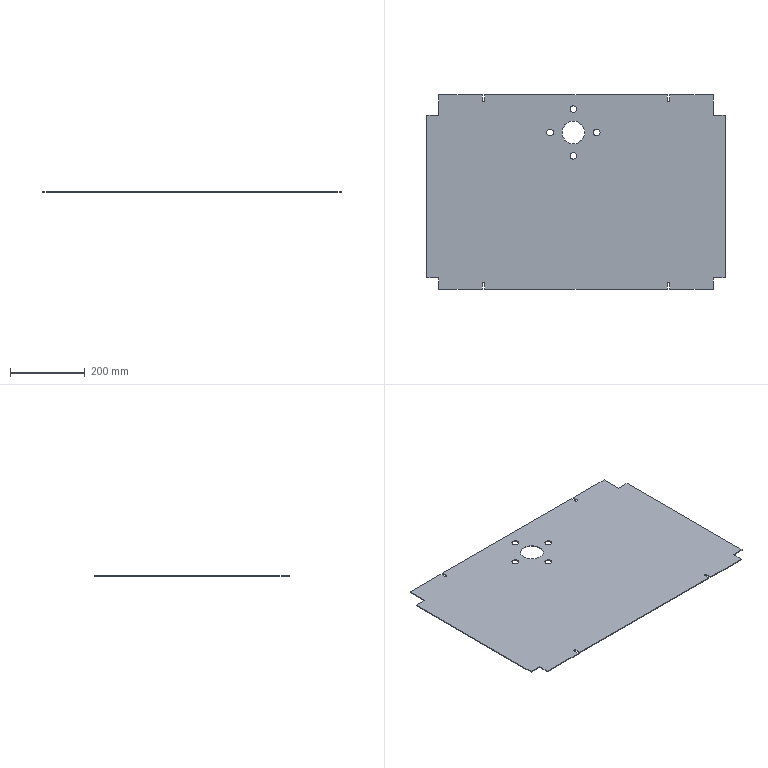Part | STEP file | JBJ-P-1006-06 | 1 solid | 35 faces | box 800 x 521 x 2 mm | volume 813927 mm3 | plane 26 | cylinder 9 | commonest cylinder face diameters 6.5 x4 18 x4 61 x1
STEP:
#1=CARTESIAN_POINT('',(155.25,-521.,2.));
#2=VERTEX_POINT('',#1);
#3=CARTESIAN_POINT('',(644.75,-521.,2.));
#4=VERTEX_POINT('',#3);
#5=CARTESIAN_POINT('',(0.,-521.,2.));
#6=DIRECTION('',(1.,0.,0.));
#7=VECTOR('',#6,1000.);
#8=LINE('',#5,#7);
#9=EDGE_CURVE('',#2,#4,#8,.T.);
#10=ORIENTED_EDGE('',*,*,#9,.F.);
#11=CARTESIAN_POINT('',(155.25,-521.,0.));
#12=VERTEX_POINT('',#11);
#13=CARTESIAN_POINT('',(155.25,-521.,2.));
#14=DIRECTION('',(0.,0.,-1.));
#15=VECTOR('',#14,1000.);
#16=LINE('',#13,#15);
#17=EDGE_CURVE('',#2,#12,#16,.T.);
#18=ORIENTED_EDGE('',*,*,#17,.T.);
#19=CARTESIAN_POINT('',(644.75,-521.,0.));
#20=VERTEX_POINT('',#19);
#21=CARTESIAN_POINT('',(0.,-521.,0.));
#22=DIRECTION('',(1.,0.,0.));
#23=VECTOR('',#22,1000.);
#24=LINE('',#21,#23);
#25=EDGE_CURVE('',#12,#20,#24,.T.);
#26=ORIENTED_EDGE('',*,*,#25,.T.);
#27=CARTESIAN_POINT('',(644.75,-521.,2.));
#28=DIRECTION('',(0.,0.,1.));
#29=VECTOR('',#28,1000.);
#30=LINE('',#27,#29);
#31=EDGE_CURVE('',#20,#4,#30,.T.);
#32=ORIENTED_EDGE('',*,*,#31,.T.);
#33=EDGE_LOOP('',(#10,#18,#26,#32));
#34=FACE_OUTER_BOUND('',#33,.T.);
#35=CARTESIAN_POINT('',(0.,-521.,2.));
#36=DIRECTION('',(0.,1.,0.));
#37=DIRECTION('',(0.,0.,1.));
#38=AXIS2_PLACEMENT_3D('',#35,#36,#37);
#39=PLANE('',#38);
#40=ADVANCED_FACE('',(#34),#39,.F.);
#41=CARTESIAN_POINT('',(651.25,-521.,2.));
#42=VERTEX_POINT('',#41);
#43=CARTESIAN_POINT('',(768.,-521.,2.));
#44=VERTEX_POINT('',#43);
#45=CARTESIAN_POINT('',(0.,-521.,2.));
#46=DIRECTION('',(1.,0.,0.));
#47=VECTOR('',#46,1000.);
#48=LINE('',#45,#47);
#49=EDGE_CURVE('',#42,#44,#48,.T.);
#50=ORIENTED_EDGE('',*,*,#49,.F.);
#51=CARTESIAN_POINT('',(651.25,-521.,0.));
#52=VERTEX_POINT('',#51);
#53=CARTESIAN_POINT('',(651.25,-521.,2.));
#54=DIRECTION('',(0.,0.,-1.));
#55=VECTOR('',#54,1000.);
#56=LINE('',#53,#55);
#57=EDGE_CURVE('',#42,#52,#56,.T.);
#58=ORIENTED_EDGE('',*,*,#57,.T.);
#59=CARTESIAN_POINT('',(768.,-521.,0.));
#60=VERTEX_POINT('',#59);
#61=CARTESIAN_POINT('',(0.,-521.,0.));
#62=DIRECTION('',(1.,0.,0.));
#63=VECTOR('',#62,1000.);
#64=LINE('',#61,#63);
#65=EDGE_CURVE('',#52,#60,#64,.T.);
#66=ORIENTED_EDGE('',*,*,#65,.T.);
#67=CARTESIAN_POINT('',(768.,-521.,3.));
#68=DIRECTION('',(0.,0.,-1.));
#69=VECTOR('',#68,1000.);
#70=LINE('',#67,#69);
#71=EDGE_CURVE('',#44,#60,#70,.T.);
#72=ORIENTED_EDGE('',*,*,#71,.F.);
#73=EDGE_LOOP('',(#50,#58,#66,#72));
#74=FACE_OUTER_BOUND('',#73,.T.);
#75=CARTESIAN_POINT('',(0.,-521.,2.));
#76=DIRECTION('',(0.,1.,0.));
#77=DIRECTION('',(0.,0.,1.));
#78=AXIS2_PLACEMENT_3D('',#75,#76,#77);
#79=PLANE('',#78);
#80=ADVANCED_FACE('',(#74),#79,.F.);
#81=CARTESIAN_POINT('',(644.75,0.,0.));
#82=VERTEX_POINT('',#81);
#83=CARTESIAN_POINT('',(644.75,0.,2.));
#84=VERTEX_POINT('',#83);
#85=CARTESIAN_POINT('',(644.75,0.,2.));
#86=DIRECTION('',(0.,0.,1.));
#87=VECTOR('',#86,1000.);
#88=LINE('',#85,#87);
#89=EDGE_CURVE('',#82,#84,#88,.T.);
#90=ORIENTED_EDGE('',*,*,#89,.F.);
#91=CARTESIAN_POINT('',(155.25,0.,0.));
#92=VERTEX_POINT('',#91);
#93=CARTESIAN_POINT('',(0.,0.,0.));
#94=DIRECTION('',(1.,0.,0.));
#95=VECTOR('',#94,1000.);
#96=LINE('',#93,#95);
#97=EDGE_CURVE('',#92,#82,#96,.T.);
#98=ORIENTED_EDGE('',*,*,#97,.F.);
#99=CARTESIAN_POINT('',(155.25,0.,2.));
#100=VERTEX_POINT('',#99);
#101=CARTESIAN_POINT('',(155.25,0.,2.));
#102=DIRECTION('',(0.,0.,-1.));
#103=VECTOR('',#102,1000.);
#104=LINE('',#101,#103);
#105=EDGE_CURVE('',#100,#92,#104,.T.);
#106=ORIENTED_EDGE('',*,*,#105,.F.);
#107=CARTESIAN_POINT('',(0.,0.,2.));
#108=DIRECTION('',(1.,0.,0.));
#109=VECTOR('',#108,1000.);
#110=LINE('',#107,#109);
#111=EDGE_CURVE('',#100,#84,#110,.T.);
#112=ORIENTED_EDGE('',*,*,#111,.T.);
#113=EDGE_LOOP('',(#90,#98,#106,#112));
#114=FACE_OUTER_BOUND('',#113,.T.);
#115=CARTESIAN_POINT('',(0.,0.,2.));
#116=DIRECTION('',(0.,1.,0.));
#117=DIRECTION('',(0.,0.,1.));
#118=AXIS2_PLACEMENT_3D('',#115,#116,#117);
#119=PLANE('',#118);
#120=ADVANCED_FACE('',(#114),#119,.T.);
#121=CARTESIAN_POINT('',(148.75,0.,0.));
#122=VERTEX_POINT('',#121);
#123=CARTESIAN_POINT('',(148.75,0.,2.));
#124=VERTEX_POINT('',#123);
#125=CARTESIAN_POINT('',(148.75,0.,2.));
#126=DIRECTION('',(0.,0.,1.));
#127=VECTOR('',#126,1000.);
#128=LINE('',#125,#127);
#129=EDGE_CURVE('',#122,#124,#128,.T.);
#130=ORIENTED_EDGE('',*,*,#129,.F.);
#131=CARTESIAN_POINT('',(32.,0.,0.));
#132=VERTEX_POINT('',#131);
#133=CARTESIAN_POINT('',(0.,0.,0.));
#134=DIRECTION('',(1.,0.,0.));
#135=VECTOR('',#134,1000.);
#136=LINE('',#133,#135);
#137=EDGE_CURVE('',#132,#122,#136,.T.);
#138=ORIENTED_EDGE('',*,*,#137,.F.);
#139=CARTESIAN_POINT('',(32.,0.,2.));
#140=VERTEX_POINT('',#139);
#141=CARTESIAN_POINT('',(32.,0.,3.));
#142=DIRECTION('',(0.,0.,-1.));
#143=VECTOR('',#142,1000.);
#144=LINE('',#141,#143);
#145=EDGE_CURVE('',#140,#132,#144,.T.);
#146=ORIENTED_EDGE('',*,*,#145,.F.);
#147=CARTESIAN_POINT('',(0.,0.,2.));
#148=DIRECTION('',(1.,0.,0.));
#149=VECTOR('',#148,1000.);
#150=LINE('',#147,#149);
#151=EDGE_CURVE('',#140,#124,#150,.T.);
#152=ORIENTED_EDGE('',*,*,#151,.T.);
#153=EDGE_LOOP('',(#130,#138,#146,#152));
#154=FACE_OUTER_BOUND('',#153,.T.);
#155=CARTESIAN_POINT('',(0.,0.,2.));
#156=DIRECTION('',(0.,1.,0.));
#157=DIRECTION('',(0.,0.,1.));
#158=AXIS2_PLACEMENT_3D('',#155,#156,#157);
#159=PLANE('',#158);
#160=ADVANCED_FACE('',(#154),#159,.T.);
#161=CARTESIAN_POINT('',(423.5,-100.992,0.));
#162=VERTEX_POINT('',#161);
#163=CARTESIAN_POINT('',(393.,-100.992,0.));
#164=DIRECTION('',(0.,0.,1.));
#165=DIRECTION('',(1.,0.,0.));
#166=AXIS2_PLACEMENT_3D('',#163,#164,#165);
#167=CIRCLE('',#166,30.5);
#168=EDGE_CURVE('',#162,#162,#167,.T.);
#169=ORIENTED_EDGE('',*,*,#168,.T.);
#170=EDGE_LOOP('',(#169));
#171=FACE_BOUND('',#170,.T.);
#172=CARTESIAN_POINT('',(384.,-163.492,0.));
#173=VERTEX_POINT('',#172);
#174=CARTESIAN_POINT('',(393.,-163.492,0.));
#175=DIRECTION('',(0.,0.,-1.));
#176=DIRECTION('',(-1.,0.,0.));
#177=AXIS2_PLACEMENT_3D('',#174,#175,#176);
#178=CIRCLE('',#177,9.);
#179=EDGE_CURVE('',#173,#173,#178,.T.);
#180=ORIENTED_EDGE('',*,*,#179,.F.);
#181=EDGE_LOOP('',(#180));
#182=FACE_BOUND('',#181,.T.);
#183=CARTESIAN_POINT('',(321.5,-100.992,0.));
#184=VERTEX_POINT('',#183);
#185=CARTESIAN_POINT('',(330.5,-100.992,0.));
#186=DIRECTION('',(0.,0.,-1.));
#187=DIRECTION('',(-1.,0.,0.));
#188=AXIS2_PLACEMENT_3D('',#185,#186,#187);
#189=CIRCLE('',#188,9.);
#190=EDGE_CURVE('',#184,#184,#189,.T.);
#191=ORIENTED_EDGE('',*,*,#190,.F.);
#192=EDGE_LOOP('',(#191));
#193=FACE_BOUND('',#192,.T.);
#194=CARTESIAN_POINT('',(384.,-38.492,0.));
#195=VERTEX_POINT('',#194);
#196=CARTESIAN_POINT('',(393.,-38.492,0.));
#197=DIRECTION('',(0.,0.,-1.));
#198=DIRECTION('',(-1.,0.,0.));
#199=AXIS2_PLACEMENT_3D('',#196,#197,#198);
#200=CIRCLE('',#199,9.);
#201=EDGE_CURVE('',#195,#195,#200,.T.);
#202=ORIENTED_EDGE('',*,*,#201,.F.);
#203=EDGE_LOOP('',(#202));
#204=FACE_BOUND('',#203,.T.);
#205=ORIENTED_EDGE('',*,*,#25,.F.);
#206=CARTESIAN_POINT('',(155.25,-506.,0.));
#207=VERTEX_POINT('',#206);
#208=CARTESIAN_POINT('',(155.25,-536.,0.));
#209=DIRECTION('',(0.,-1.,0.));
#210=VECTOR('',#209,1000.);
#211=LINE('',#208,#210);
#212=EDGE_CURVE('',#207,#12,#211,.T.);
#213=ORIENTED_EDGE('',*,*,#212,.F.);
#214=CARTESIAN_POINT('',(148.75,-506.,0.));
#215=VERTEX_POINT('',#214);
#216=CARTESIAN_POINT('',(152.,-506.,0.));
#217=DIRECTION('',(0.,0.,-1.));
#218=DIRECTION('',(1.,0.,0.));
#219=AXIS2_PLACEMENT_3D('',#216,#217,#218);
#220=CIRCLE('',#219,3.25);
#221=EDGE_CURVE('',#215,#207,#220,.T.);
#222=ORIENTED_EDGE('',*,*,#221,.F.);
#223=CARTESIAN_POINT('',(148.75,-521.,0.));
#224=VERTEX_POINT('',#223);
#225=CARTESIAN_POINT('',(148.75,-536.,0.));
#226=DIRECTION('',(0.,1.,0.));
#227=VECTOR('',#226,1000.);
#228=LINE('',#225,#227);
#229=EDGE_CURVE('',#224,#215,#228,.T.);
#230=ORIENTED_EDGE('',*,*,#229,.F.);
#231=CARTESIAN_POINT('',(32.,-521.,0.));
#232=VERTEX_POINT('',#231);
#233=CARTESIAN_POINT('',(0.,-521.,0.));
#234=DIRECTION('',(1.,0.,0.));
#235=VECTOR('',#234,1000.);
#236=LINE('',#233,#235);
#237=EDGE_CURVE('',#232,#224,#236,.T.);
#238=ORIENTED_EDGE('',*,*,#237,.F.);
#239=CARTESIAN_POINT('',(32.,-491.,0.));
#240=VERTEX_POINT('',#239);
#241=CARTESIAN_POINT('',(32.,-521.,0.));
#242=DIRECTION('',(0.,-1.,0.));
#243=VECTOR('',#242,1000.);
#244=LINE('',#241,#243);
#245=EDGE_CURVE('',#240,#232,#244,.T.);
#246=ORIENTED_EDGE('',*,*,#245,.F.);
#247=CARTESIAN_POINT('',(0.,-491.,0.));
#248=VERTEX_POINT('',#247);
#249=CARTESIAN_POINT('',(0.,-491.,0.));
#250=DIRECTION('',(1.,0.,0.));
#251=VECTOR('',#250,1000.);
#252=LINE('',#249,#251);
#253=EDGE_CURVE('',#248,#240,#252,.T.);
#254=ORIENTED_EDGE('',*,*,#253,.F.);
#255=CARTESIAN_POINT('',(0.,-55.,0.));
#256=VERTEX_POINT('',#255);
#257=CARTESIAN_POINT('',(0.,0.,0.));
#258=DIRECTION('',(0.,-1.,0.));
#259=VECTOR('',#258,1000.);
#260=LINE('',#257,#259);
#261=EDGE_CURVE('',#256,#248,#260,.T.);
#262=ORIENTED_EDGE('',*,*,#261,.F.);
#263=CARTESIAN_POINT('',(32.,-55.,0.));
#264=VERTEX_POINT('',#263);
#265=CARTESIAN_POINT('',(0.,-55.,0.));
#266=DIRECTION('',(-1.,0.,0.));
#267=VECTOR('',#266,1000.);
#268=LINE('',#265,#267);
#269=EDGE_CURVE('',#264,#256,#268,.T.);
#270=ORIENTED_EDGE('',*,*,#269,.F.);
#271=CARTESIAN_POINT('',(32.,0.,0.));
#272=DIRECTION('',(0.,-1.,0.));
#273=VECTOR('',#272,1000.);
#274=LINE('',#271,#273);
#275=EDGE_CURVE('',#132,#264,#274,.T.);
#276=ORIENTED_EDGE('',*,*,#275,.F.);
#277=ORIENTED_EDGE('',*,*,#137,.T.);
#278=CARTESIAN_POINT('',(148.75,-15.,0.));
#279=VERTEX_POINT('',#278);
#280=CARTESIAN_POINT('',(148.75,15.,0.));
#281=DIRECTION('',(0.,1.,0.));
#282=VECTOR('',#281,1000.);
#283=LINE('',#280,#282);
#284=EDGE_CURVE('',#279,#122,#283,.T.);
#285=ORIENTED_EDGE('',*,*,#284,.F.);
#286=CARTESIAN_POINT('',(155.25,-15.,0.));
#287=VERTEX_POINT('',#286);
#288=CARTESIAN_POINT('',(152.,-15.,0.));
#289=DIRECTION('',(0.,0.,-1.));
#290=DIRECTION('',(-1.,0.,0.));
#291=AXIS2_PLACEMENT_3D('',#288,#289,#290);
#292=CIRCLE('',#291,3.25);
#293=EDGE_CURVE('',#287,#279,#292,.T.);
#294=ORIENTED_EDGE('',*,*,#293,.F.);
#295=CARTESIAN_POINT('',(155.25,15.,0.));
#296=DIRECTION('',(0.,-1.,0.));
#297=VECTOR('',#296,1000.);
#298=LINE('',#295,#297);
#299=EDGE_CURVE('',#92,#287,#298,.T.);
#300=ORIENTED_EDGE('',*,*,#299,.F.);
#301=ORIENTED_EDGE('',*,*,#97,.T.);
#302=CARTESIAN_POINT('',(644.75,-15.,0.));
#303=VERTEX_POINT('',#302);
#304=CARTESIAN_POINT('',(644.75,15.,0.));
#305=DIRECTION('',(0.,1.,0.));
#306=VECTOR('',#305,1000.);
#307=LINE('',#304,#306);
#308=EDGE_CURVE('',#303,#82,#307,.T.);
#309=ORIENTED_EDGE('',*,*,#308,.F.);
#310=CARTESIAN_POINT('',(651.25,-15.,0.));
#311=VERTEX_POINT('',#310);
#312=CARTESIAN_POINT('',(648.,-15.,0.));
#313=DIRECTION('',(0.,0.,-1.));
#314=DIRECTION('',(1.,0.,0.));
#315=AXIS2_PLACEMENT_3D('',#312,#313,#314);
#316=CIRCLE('',#315,3.25);
#317=EDGE_CURVE('',#311,#303,#316,.T.);
#318=ORIENTED_EDGE('',*,*,#317,.F.);
#319=CARTESIAN_POINT('',(651.25,0.,0.));
#320=VERTEX_POINT('',#319);
#321=CARTESIAN_POINT('',(651.25,15.,0.));
#322=DIRECTION('',(0.,-1.,0.));
#323=VECTOR('',#322,1000.);
#324=LINE('',#321,#323);
#325=EDGE_CURVE('',#320,#311,#324,.T.);
#326=ORIENTED_EDGE('',*,*,#325,.F.);
#327=CARTESIAN_POINT('',(768.,0.,0.));
#328=VERTEX_POINT('',#327);
#329=CARTESIAN_POINT('',(0.,0.,0.));
#330=DIRECTION('',(1.,0.,0.));
#331=VECTOR('',#330,1000.);
#332=LINE('',#329,#331);
#333=EDGE_CURVE('',#320,#328,#332,.T.);
#334=ORIENTED_EDGE('',*,*,#333,.T.);
#335=CARTESIAN_POINT('',(768.,-55.,0.));
#336=VERTEX_POINT('',#335);
#337=CARTESIAN_POINT('',(768.,0.,0.));
#338=DIRECTION('',(0.,1.,0.));
#339=VECTOR('',#338,1000.);
#340=LINE('',#337,#339);
#341=EDGE_CURVE('',#336,#328,#340,.T.);
#342=ORIENTED_EDGE('',*,*,#341,.F.);
#343=CARTESIAN_POINT('',(800.,-55.,0.));
#344=VERTEX_POINT('',#343);
#345=CARTESIAN_POINT('',(800.,-55.,0.));
#346=DIRECTION('',(-1.,0.,0.));
#347=VECTOR('',#346,1000.);
#348=LINE('',#345,#347);
#349=EDGE_CURVE('',#344,#336,#348,.T.);
#350=ORIENTED_EDGE('',*,*,#349,.F.);
#351=CARTESIAN_POINT('',(800.,-491.,0.));
#352=VERTEX_POINT('',#351);
#353=CARTESIAN_POINT('',(800.,0.,0.));
#354=DIRECTION('',(0.,-1.,0.));
#355=VECTOR('',#354,1000.);
#356=LINE('',#353,#355);
#357=EDGE_CURVE('',#344,#352,#356,.T.);
#358=ORIENTED_EDGE('',*,*,#357,.T.);
#359=CARTESIAN_POINT('',(768.,-491.,0.));
#360=VERTEX_POINT('',#359);
#361=CARTESIAN_POINT('',(800.,-491.,0.));
#362=DIRECTION('',(1.,0.,0.));
#363=VECTOR('',#362,1000.);
#364=LINE('',#361,#363);
#365=EDGE_CURVE('',#360,#352,#364,.T.);
#366=ORIENTED_EDGE('',*,*,#365,.F.);
#367=CARTESIAN_POINT('',(768.,-521.,0.));
#368=DIRECTION('',(0.,1.,0.));
#369=VECTOR('',#368,1000.);
#370=LINE('',#367,#369);
#371=EDGE_CURVE('',#60,#360,#370,.T.);
#372=ORIENTED_EDGE('',*,*,#371,.F.);
#373=ORIENTED_EDGE('',*,*,#65,.F.);
#374=CARTESIAN_POINT('',(651.25,-506.,0.));
#375=VERTEX_POINT('',#374);
#376=CARTESIAN_POINT('',(651.25,-536.,0.));
#377=DIRECTION('',(0.,-1.,0.));
#378=VECTOR('',#377,1000.);
#379=LINE('',#376,#378);
#380=EDGE_CURVE('',#375,#52,#379,.T.);
#381=ORIENTED_EDGE('',*,*,#380,.F.);
#382=CARTESIAN_POINT('',(644.75,-506.,0.));
#383=VERTEX_POINT('',#382);
#384=CARTESIAN_POINT('',(648.,-506.,0.));
#385=DIRECTION('',(0.,0.,-1.));
#386=DIRECTION('',(-1.,0.,0.));
#387=AXIS2_PLACEMENT_3D('',#384,#385,#386);
#388=CIRCLE('',#387,3.25);
#389=EDGE_CURVE('',#383,#375,#388,.T.);
#390=ORIENTED_EDGE('',*,*,#389,.F.);
#391=CARTESIAN_POINT('',(644.75,-536.,0.));
#392=DIRECTION('',(0.,1.,0.));
#393=VECTOR('',#392,1000.);
#394=LINE('',#391,#393);
#395=EDGE_CURVE('',#20,#383,#394,.T.);
#396=ORIENTED_EDGE('',*,*,#395,.F.);
#397=EDGE_LOOP('',(#205,#213,#222,#230,#238,#246,#254,#262,#270,#276,#277,#285,#294,#300,#301,#309,#318,#326,#334,#342,#350,#358,#366,#372,#373,#381,#390,#396));
#398=FACE_OUTER_BOUND('',#397,.T.);
#399=CARTESIAN_POINT('',(446.5,-100.992,0.));
#400=VERTEX_POINT('',#399);
#401=CARTESIAN_POINT('',(455.5,-100.992,0.));
#402=DIRECTION('',(0.,0.,-1.));
#403=DIRECTION('',(-1.,0.,0.));
#404=AXIS2_PLACEMENT_3D('',#401,#402,#403);
#405=CIRCLE('',#404,9.);
#406=EDGE_CURVE('',#400,#400,#405,.T.);
#407=ORIENTED_EDGE('',*,*,#406,.F.);
#408=EDGE_LOOP('',(#407));
#409=FACE_BOUND('',#408,.T.);
#410=CARTESIAN_POINT('',(0.,0.,0.));
#411=DIRECTION('',(0.,0.,1.));
#412=DIRECTION('',(1.,0.,0.));
#413=AXIS2_PLACEMENT_3D('',#410,#411,#412);
#414=PLANE('',#413);
#415=ADVANCED_FACE('',(#171,#182,#193,#204,#398,#409),#414,.F.);
#416=ORIENTED_EDGE('',*,*,#261,.T.);
#417=CARTESIAN_POINT('',(0.,-491.,2.));
#418=VERTEX_POINT('',#417);
#419=CARTESIAN_POINT('',(0.,-491.,3.));
#420=DIRECTION('',(0.,0.,-1.));
#421=VECTOR('',#420,1000.);
#422=LINE('',#419,#421);
#423=EDGE_CURVE('',#418,#248,#422,.T.);
#424=ORIENTED_EDGE('',*,*,#423,.F.);
#425=CARTESIAN_POINT('',(0.,-55.,2.));
#426=VERTEX_POINT('',#425);
#427=CARTESIAN_POINT('',(0.,0.,2.));
#428=DIRECTION('',(0.,-1.,0.));
#429=VECTOR('',#428,1000.);
#430=LINE('',#427,#429);
#431=EDGE_CURVE('',#426,#418,#430,.T.);
#432=ORIENTED_EDGE('',*,*,#431,.F.);
#433=CARTESIAN_POINT('',(0.,-55.,3.));
#434=DIRECTION('',(0.,0.,-1.));
#435=VECTOR('',#434,1000.);
#436=LINE('',#433,#435);
#437=EDGE_CURVE('',#426,#256,#436,.T.);
#438=ORIENTED_EDGE('',*,*,#437,.T.);
#439=EDGE_LOOP('',(#416,#424,#432,#438));
#440=FACE_OUTER_BOUND('',#439,.T.);
#441=CARTESIAN_POINT('',(0.,0.,2.));
#442=DIRECTION('',(1.,0.,0.));
#443=DIRECTION('',(0.,1.,0.));
#444=AXIS2_PLACEMENT_3D('',#441,#442,#443);
#445=PLANE('',#444);
#446=ADVANCED_FACE('',(#440),#445,.F.);
#447=ORIENTED_EDGE('',*,*,#237,.T.);
#448=CARTESIAN_POINT('',(148.75,-521.,2.));
#449=VERTEX_POINT('',#448);
#450=CARTESIAN_POINT('',(148.75,-521.,2.));
#451=DIRECTION('',(0.,0.,1.));
#452=VECTOR('',#451,1000.);
#453=LINE('',#450,#452);
#454=EDGE_CURVE('',#224,#449,#453,.T.);
#455=ORIENTED_EDGE('',*,*,#454,.T.);
#456=CARTESIAN_POINT('',(32.,-521.,2.));
#457=VERTEX_POINT('',#456);
#458=CARTESIAN_POINT('',(0.,-521.,2.));
#459=DIRECTION('',(1.,0.,0.));
#460=VECTOR('',#459,1000.);
#461=LINE('',#458,#460);
#462=EDGE_CURVE('',#457,#449,#461,.T.);
#463=ORIENTED_EDGE('',*,*,#462,.F.);
#464=CARTESIAN_POINT('',(32.,-521.,3.));
#465=DIRECTION('',(0.,0.,-1.));
#466=VECTOR('',#465,1000.);
#467=LINE('',#464,#466);
#468=EDGE_CURVE('',#457,#232,#467,.T.);
#469=ORIENTED_EDGE('',*,*,#468,.T.);
#470=EDGE_LOOP('',(#447,#455,#463,#469));
#471=FACE_OUTER_BOUND('',#470,.T.);
#472=CARTESIAN_POINT('',(0.,-521.,2.));
#473=DIRECTION('',(0.,1.,0.));
#474=DIRECTION('',(0.,0.,1.));
#475=AXIS2_PLACEMENT_3D('',#472,#473,#474);
#476=PLANE('',#475);
#477=ADVANCED_FACE('',(#471),#476,.F.);
#478=CARTESIAN_POINT('',(800.,-55.,2.));
#479=VERTEX_POINT('',#478);
#480=CARTESIAN_POINT('',(800.,-55.,3.));
#481=DIRECTION('',(0.,0.,-1.));
#482=VECTOR('',#481,1000.);
#483=LINE('',#480,#482);
#484=EDGE_CURVE('',#479,#344,#483,.T.);
#485=ORIENTED_EDGE('',*,*,#484,.F.);
#486=CARTESIAN_POINT('',(800.,-491.,2.));
#487=VERTEX_POINT('',#486);
#488=CARTESIAN_POINT('',(800.,0.,2.));
#489=DIRECTION('',(0.,-1.,0.));
#490=VECTOR('',#489,1000.);
#491=LINE('',#488,#490);
#492=EDGE_CURVE('',#479,#487,#491,.T.);
#493=ORIENTED_EDGE('',*,*,#492,.T.);
#494=CARTESIAN_POINT('',(800.,-491.,3.));
#495=DIRECTION('',(0.,0.,-1.));
#496=VECTOR('',#495,1000.);
#497=LINE('',#494,#496);
#498=EDGE_CURVE('',#487,#352,#497,.T.);
#499=ORIENTED_EDGE('',*,*,#498,.T.);
#500=ORIENTED_EDGE('',*,*,#357,.F.);
#501=EDGE_LOOP('',(#485,#493,#499,#500));
#502=FACE_OUTER_BOUND('',#501,.T.);
#503=CARTESIAN_POINT('',(800.,0.,2.));
#504=DIRECTION('',(1.,0.,0.));
#505=DIRECTION('',(0.,1.,0.));
#506=AXIS2_PLACEMENT_3D('',#503,#504,#505);
#507=PLANE('',#506);
#508=ADVANCED_FACE('',(#502),#507,.T.);
#509=CARTESIAN_POINT('',(651.25,0.,2.));
#510=VERTEX_POINT('',#509);
#511=CARTESIAN_POINT('',(651.25,0.,2.));
#512=DIRECTION('',(0.,0.,-1.));
#513=VECTOR('',#512,1000.);
#514=LINE('',#511,#513);
#515=EDGE_CURVE('',#510,#320,#514,.T.);
#516=ORIENTED_EDGE('',*,*,#515,.F.);
#517=CARTESIAN_POINT('',(768.,0.,2.));
#518=VERTEX_POINT('',#517);
#519=CARTESIAN_POINT('',(0.,0.,2.));
#520=DIRECTION('',(1.,0.,0.));
#521=VECTOR('',#520,1000.);
#522=LINE('',#519,#521);
#523=EDGE_CURVE('',#510,#518,#522,.T.);
#524=ORIENTED_EDGE('',*,*,#523,.T.);
#525=CARTESIAN_POINT('',(768.,0.,3.));
#526=DIRECTION('',(0.,0.,-1.));
#527=VECTOR('',#526,1000.);
#528=LINE('',#525,#527);
#529=EDGE_CURVE('',#518,#328,#528,.T.);
#530=ORIENTED_EDGE('',*,*,#529,.T.);
#531=ORIENTED_EDGE('',*,*,#333,.F.);
#532=EDGE_LOOP('',(#516,#524,#530,#531));
#533=FACE_OUTER_BOUND('',#532,.T.);
#534=CARTESIAN_POINT('',(0.,0.,2.));
#535=DIRECTION('',(0.,1.,0.));
#536=DIRECTION('',(0.,0.,1.));
#537=AXIS2_PLACEMENT_3D('',#534,#535,#536);
#538=PLANE('',#537);
#539=ADVANCED_FACE('',(#533),#538,.T.);
#540=CARTESIAN_POINT('',(155.25,-506.,2.));
#541=VERTEX_POINT('',#540);
#542=CARTESIAN_POINT('',(155.25,0.,2.));
#543=DIRECTION('',(0.,1.,0.));
#544=VECTOR('',#543,1000.);
#545=LINE('',#542,#544);
#546=EDGE_CURVE('',#2,#541,#545,.T.);
#547=ORIENTED_EDGE('',*,*,#546,.F.);
#548=ORIENTED_EDGE('',*,*,#9,.T.);
#549=CARTESIAN_POINT('',(644.75,-506.,2.));
#550=VERTEX_POINT('',#549);
#551=CARTESIAN_POINT('',(644.75,0.,2.));
#552=DIRECTION('',(0.,-1.,0.));
#553=VECTOR('',#552,1000.);
#554=LINE('',#551,#553);
#555=EDGE_CURVE('',#550,#4,#554,.T.);
#556=ORIENTED_EDGE('',*,*,#555,.F.);
#557=CARTESIAN_POINT('',(651.25,-506.,2.));
#558=VERTEX_POINT('',#557);
#559=CARTESIAN_POINT('',(648.,-506.,2.));
#560=DIRECTION('',(0.,0.,1.));
#561=DIRECTION('',(1.,0.,0.));
#562=AXIS2_PLACEMENT_3D('',#559,#560,#561);
#563=CIRCLE('',#562,3.25);
#564=EDGE_CURVE('',#558,#550,#563,.T.);
#565=ORIENTED_EDGE('',*,*,#564,.F.);
#566=CARTESIAN_POINT('',(651.25,0.,2.));
#567=DIRECTION('',(0.,1.,0.));
#568=VECTOR('',#567,1000.);
#569=LINE('',#566,#568);
#570=EDGE_CURVE('',#42,#558,#569,.T.);
#571=ORIENTED_EDGE('',*,*,#570,.F.);
#572=ORIENTED_EDGE('',*,*,#49,.T.);
#573=CARTESIAN_POINT('',(768.,-491.,2.));
#574=VERTEX_POINT('',#573);
#575=CARTESIAN_POINT('',(768.,0.,2.));
#576=DIRECTION('',(0.,-1.,0.));
#577=VECTOR('',#576,1000.);
#578=LINE('',#575,#577);
#579=EDGE_CURVE('',#574,#44,#578,.T.);
#580=ORIENTED_EDGE('',*,*,#579,.F.);
#581=CARTESIAN_POINT('',(0.,-491.,2.));
#582=DIRECTION('',(-1.,0.,0.));
#583=VECTOR('',#582,1000.);
#584=LINE('',#581,#583);
#585=EDGE_CURVE('',#487,#574,#584,.T.);
#586=ORIENTED_EDGE('',*,*,#585,.F.);
#587=ORIENTED_EDGE('',*,*,#492,.F.);
#588=CARTESIAN_POINT('',(768.,-55.,2.));
#589=VERTEX_POINT('',#588);
#590=CARTESIAN_POINT('',(0.,-55.,2.));
#591=DIRECTION('',(1.,0.,0.));
#592=VECTOR('',#591,1000.);
#593=LINE('',#590,#592);
#594=EDGE_CURVE('',#589,#479,#593,.T.);
#595=ORIENTED_EDGE('',*,*,#594,.F.);
#596=CARTESIAN_POINT('',(768.,0.,2.));
#597=DIRECTION('',(0.,-1.,0.));
#598=VECTOR('',#597,1000.);
#599=LINE('',#596,#598);
#600=EDGE_CURVE('',#518,#589,#599,.T.);
#601=ORIENTED_EDGE('',*,*,#600,.F.);
#602=ORIENTED_EDGE('',*,*,#523,.F.);
#603=CARTESIAN_POINT('',(651.25,-15.,2.));
#604=VERTEX_POINT('',#603);
#605=CARTESIAN_POINT('',(651.25,0.,2.));
#606=DIRECTION('',(0.,1.,0.));
#607=VECTOR('',#606,1000.);
#608=LINE('',#605,#607);
#609=EDGE_CURVE('',#604,#510,#608,.T.);
#610=ORIENTED_EDGE('',*,*,#609,.F.);
#611=CARTESIAN_POINT('',(644.75,-15.,2.));
#612=VERTEX_POINT('',#611);
#613=CARTESIAN_POINT('',(648.,-15.,2.));
#614=DIRECTION('',(0.,0.,1.));
#615=DIRECTION('',(1.,0.,0.));
#616=AXIS2_PLACEMENT_3D('',#613,#614,#615);
#617=CIRCLE('',#616,3.25);
#618=EDGE_CURVE('',#612,#604,#617,.T.);
#619=ORIENTED_EDGE('',*,*,#618,.F.);
#620=CARTESIAN_POINT('',(644.75,0.,2.));
#621=DIRECTION('',(0.,-1.,0.));
#622=VECTOR('',#621,1000.);
#623=LINE('',#620,#622);
#624=EDGE_CURVE('',#84,#612,#623,.T.);
#625=ORIENTED_EDGE('',*,*,#624,.F.);
#626=ORIENTED_EDGE('',*,*,#111,.F.);
#627=CARTESIAN_POINT('',(155.25,-15.,2.));
#628=VERTEX_POINT('',#627);
#629=CARTESIAN_POINT('',(155.25,0.,2.));
#630=DIRECTION('',(0.,1.,0.));
#631=VECTOR('',#630,1000.);
#632=LINE('',#629,#631);
#633=EDGE_CURVE('',#628,#100,#632,.T.);
#634=ORIENTED_EDGE('',*,*,#633,.F.);
#635=CARTESIAN_POINT('',(148.75,-15.,2.));
#636=VERTEX_POINT('',#635);
#637=CARTESIAN_POINT('',(152.,-15.,2.));
#638=DIRECTION('',(0.,0.,1.));
#639=DIRECTION('',(1.,0.,0.));
#640=AXIS2_PLACEMENT_3D('',#637,#638,#639);
#641=CIRCLE('',#640,3.25);
#642=EDGE_CURVE('',#636,#628,#641,.T.);
#643=ORIENTED_EDGE('',*,*,#642,.F.);
#644=CARTESIAN_POINT('',(148.75,0.,2.));
#645=DIRECTION('',(0.,-1.,0.));
#646=VECTOR('',#645,1000.);
#647=LINE('',#644,#646);
#648=EDGE_CURVE('',#124,#636,#647,.T.);
#649=ORIENTED_EDGE('',*,*,#648,.F.);
#650=ORIENTED_EDGE('',*,*,#151,.F.);
#651=CARTESIAN_POINT('',(32.,-55.,2.));
#652=VERTEX_POINT('',#651);
#653=CARTESIAN_POINT('',(32.,0.,2.));
#654=DIRECTION('',(0.,1.,0.));
#655=VECTOR('',#654,1000.);
#656=LINE('',#653,#655);
#657=EDGE_CURVE('',#652,#140,#656,.T.);
#658=ORIENTED_EDGE('',*,*,#657,.F.);
#659=CARTESIAN_POINT('',(0.,-55.,2.));
#660=DIRECTION('',(1.,0.,0.));
#661=VECTOR('',#660,1000.);
#662=LINE('',#659,#661);
#663=EDGE_CURVE('',#426,#652,#662,.T.);
#664=ORIENTED_EDGE('',*,*,#663,.F.);
#665=ORIENTED_EDGE('',*,*,#431,.T.);
#666=CARTESIAN_POINT('',(32.,-491.,2.));
#667=VERTEX_POINT('',#666);
#668=CARTESIAN_POINT('',(0.,-491.,2.));
#669=DIRECTION('',(-1.,0.,0.));
#670=VECTOR('',#669,1000.);
#671=LINE('',#668,#670);
#672=EDGE_CURVE('',#667,#418,#671,.T.);
#673=ORIENTED_EDGE('',*,*,#672,.F.);
#674=CARTESIAN_POINT('',(32.,0.,2.));
#675=DIRECTION('',(0.,1.,0.));
#676=VECTOR('',#675,1000.);
#677=LINE('',#674,#676);
#678=EDGE_CURVE('',#457,#667,#677,.T.);
#679=ORIENTED_EDGE('',*,*,#678,.F.);
#680=ORIENTED_EDGE('',*,*,#462,.T.);
#681=CARTESIAN_POINT('',(148.75,-506.,2.));
#682=VERTEX_POINT('',#681);
#683=CARTESIAN_POINT('',(148.75,0.,2.));
#684=DIRECTION('',(0.,-1.,0.));
#685=VECTOR('',#684,1000.);
#686=LINE('',#683,#685);
#687=EDGE_CURVE('',#682,#449,#686,.T.);
#688=ORIENTED_EDGE('',*,*,#687,.F.);
#689=CARTESIAN_POINT('',(152.,-506.,2.));
#690=DIRECTION('',(0.,0.,1.));
#691=DIRECTION('',(1.,0.,0.));
#692=AXIS2_PLACEMENT_3D('',#689,#690,#691);
#693=CIRCLE('',#692,3.25);
#694=EDGE_CURVE('',#541,#682,#693,.T.);
#695=ORIENTED_EDGE('',*,*,#694,.F.);
#696=EDGE_LOOP('',(#547,#548,#556,#565,#571,#572,#580,#586,#587,#595,#601,#602,#610,#619,#625,#626,#634,#643,#649,#650,#658,#664,#665,#673,#679,#680,#688,#695));
#697=FACE_OUTER_BOUND('',#696,.T.);
#698=CARTESIAN_POINT('',(423.5,-100.992,2.));
#699=VERTEX_POINT('',#698);
#700=CARTESIAN_POINT('',(393.,-100.992,2.));
#701=DIRECTION('',(0.,0.,1.));
#702=DIRECTION('',(1.,0.,0.));
#703=AXIS2_PLACEMENT_3D('',#700,#701,#702);
#704=CIRCLE('',#703,30.5);
#705=EDGE_CURVE('',#699,#699,#704,.T.);
#706=ORIENTED_EDGE('',*,*,#705,.F.);
#707=EDGE_LOOP('',(#706));
#708=FACE_BOUND('',#707,.T.);
#709=CARTESIAN_POINT('',(384.,-163.492,2.));
#710=VERTEX_POINT('',#709);
#711=CARTESIAN_POINT('',(393.,-163.492,2.));
#712=DIRECTION('',(0.,0.,-1.));
#713=DIRECTION('',(-1.,0.,0.));
#714=AXIS2_PLACEMENT_3D('',#711,#712,#713);
#715=CIRCLE('',#714,9.);
#716=EDGE_CURVE('',#710,#710,#715,.T.);
#717=ORIENTED_EDGE('',*,*,#716,.T.);
#718=EDGE_LOOP('',(#717));
#719=FACE_BOUND('',#718,.T.);
#720=CARTESIAN_POINT('',(321.5,-100.992,2.));
#721=VERTEX_POINT('',#720);
#722=CARTESIAN_POINT('',(330.5,-100.992,2.));
#723=DIRECTION('',(0.,0.,-1.));
#724=DIRECTION('',(-1.,0.,0.));
#725=AXIS2_PLACEMENT_3D('',#722,#723,#724);
#726=CIRCLE('',#725,9.);
#727=EDGE_CURVE('',#721,#721,#726,.T.);
#728=ORIENTED_EDGE('',*,*,#727,.T.);
#729=EDGE_LOOP('',(#728));
#730=FACE_BOUND('',#729,.T.);
#731=CARTESIAN_POINT('',(384.,-38.492,2.));
#732=VERTEX_POINT('',#731);
#733=CARTESIAN_POINT('',(393.,-38.492,2.));
#734=DIRECTION('',(0.,0.,-1.));
#735=DIRECTION('',(-1.,0.,0.));
#736=AXIS2_PLACEMENT_3D('',#733,#734,#735);
#737=CIRCLE('',#736,9.);
#738=EDGE_CURVE('',#732,#732,#737,.T.);
#739=ORIENTED_EDGE('',*,*,#738,.T.);
#740=EDGE_LOOP('',(#739));
#741=FACE_BOUND('',#740,.T.);
#742=CARTESIAN_POINT('',(446.5,-100.992,2.));
#743=VERTEX_POINT('',#742);
#744=CARTESIAN_POINT('',(455.5,-100.992,2.));
#745=DIRECTION('',(0.,0.,-1.));
#746=DIRECTION('',(-1.,0.,0.));
#747=AXIS2_PLACEMENT_3D('',#744,#745,#746);
#748=CIRCLE('',#747,9.);
#749=EDGE_CURVE('',#743,#743,#748,.T.);
#750=ORIENTED_EDGE('',*,*,#749,.T.);
#751=EDGE_LOOP('',(#750));
#752=FACE_BOUND('',#751,.T.);
#753=CARTESIAN_POINT('',(0.,0.,2.));
#754=DIRECTION('',(0.,0.,1.));
#755=DIRECTION('',(1.,0.,0.));
#756=AXIS2_PLACEMENT_3D('',#753,#754,#755);
#757=PLANE('',#756);
#758=ADVANCED_FACE('',(#697,#708,#719,#730,#741,#752),#757,.T.);
#759=ORIENTED_EDGE('',*,*,#663,.T.);
#760=CARTESIAN_POINT('',(32.,-55.,3.));
#761=DIRECTION('',(0.,0.,-1.));
#762=VECTOR('',#761,1000.);
#763=LINE('',#760,#762);
#764=EDGE_CURVE('',#652,#264,#763,.T.);
#765=ORIENTED_EDGE('',*,*,#764,.T.);
#766=ORIENTED_EDGE('',*,*,#269,.T.);
#767=ORIENTED_EDGE('',*,*,#437,.F.);
#768=EDGE_LOOP('',(#759,#765,#766,#767));
#769=FACE_OUTER_BOUND('',#768,.T.);
#770=CARTESIAN_POINT('',(0.,-55.,3.));
#771=DIRECTION('',(0.,-1.,0.));
#772=DIRECTION('',(0.,0.,-1.));
#773=AXIS2_PLACEMENT_3D('',#770,#771,#772);
#774=PLANE('',#773);
#775=ADVANCED_FACE('',(#769),#774,.F.);
#776=ORIENTED_EDGE('',*,*,#657,.T.);
#777=ORIENTED_EDGE('',*,*,#145,.T.);
#778=ORIENTED_EDGE('',*,*,#275,.T.);
#779=ORIENTED_EDGE('',*,*,#764,.F.);
#780=EDGE_LOOP('',(#776,#777,#778,#779));
#781=FACE_OUTER_BOUND('',#780,.T.);
#782=CARTESIAN_POINT('',(32.,0.,3.));
#783=DIRECTION('',(1.,0.,0.));
#784=DIRECTION('',(0.,1.,0.));
#785=AXIS2_PLACEMENT_3D('',#782,#783,#784);
#786=PLANE('',#785);
#787=ADVANCED_FACE('',(#781),#786,.F.);
#788=ORIENTED_EDGE('',*,*,#678,.T.);
#789=CARTESIAN_POINT('',(32.,-491.,3.));
#790=DIRECTION('',(0.,0.,-1.));
#791=VECTOR('',#790,1000.);
#792=LINE('',#789,#791);
#793=EDGE_CURVE('',#667,#240,#792,.T.);
#794=ORIENTED_EDGE('',*,*,#793,.T.);
#795=ORIENTED_EDGE('',*,*,#245,.T.);
#796=ORIENTED_EDGE('',*,*,#468,.F.);
#797=EDGE_LOOP('',(#788,#794,#795,#796));
#798=FACE_OUTER_BOUND('',#797,.T.);
#799=CARTESIAN_POINT('',(32.,-521.,3.));
#800=DIRECTION('',(1.,0.,0.));
#801=DIRECTION('',(0.,1.,0.));
#802=AXIS2_PLACEMENT_3D('',#799,#800,#801);
#803=PLANE('',#802);
#804=ADVANCED_FACE('',(#798),#803,.F.);
#805=ORIENTED_EDGE('',*,*,#672,.T.);
#806=ORIENTED_EDGE('',*,*,#423,.T.);
#807=ORIENTED_EDGE('',*,*,#253,.T.);
#808=ORIENTED_EDGE('',*,*,#793,.F.);
#809=EDGE_LOOP('',(#805,#806,#807,#808));
#810=FACE_OUTER_BOUND('',#809,.T.);
#811=CARTESIAN_POINT('',(0.,-491.,3.));
#812=DIRECTION('',(0.,1.,0.));
#813=DIRECTION('',(0.,0.,1.));
#814=AXIS2_PLACEMENT_3D('',#811,#812,#813);
#815=PLANE('',#814);
#816=ADVANCED_FACE('',(#810),#815,.F.);
#817=ORIENTED_EDGE('',*,*,#585,.T.);
#818=CARTESIAN_POINT('',(768.,-491.,3.));
#819=DIRECTION('',(0.,0.,-1.));
#820=VECTOR('',#819,1000.);
#821=LINE('',#818,#820);
#822=EDGE_CURVE('',#574,#360,#821,.T.);
#823=ORIENTED_EDGE('',*,*,#822,.T.);
#824=ORIENTED_EDGE('',*,*,#365,.T.);
#825=ORIENTED_EDGE('',*,*,#498,.F.);
#826=EDGE_LOOP('',(#817,#823,#824,#825));
#827=FACE_OUTER_BOUND('',#826,.T.);
#828=CARTESIAN_POINT('',(800.,-491.,3.));
#829=DIRECTION('',(0.,1.,0.));
#830=DIRECTION('',(0.,0.,1.));
#831=AXIS2_PLACEMENT_3D('',#828,#829,#830);
#832=PLANE('',#831);
#833=ADVANCED_FACE('',(#827),#832,.F.);
#834=ORIENTED_EDGE('',*,*,#579,.T.);
#835=ORIENTED_EDGE('',*,*,#71,.T.);
#836=ORIENTED_EDGE('',*,*,#371,.T.);
#837=ORIENTED_EDGE('',*,*,#822,.F.);
#838=EDGE_LOOP('',(#834,#835,#836,#837));
#839=FACE_OUTER_BOUND('',#838,.T.);
#840=CARTESIAN_POINT('',(768.,-521.,3.));
#841=DIRECTION('',(-1.,0.,0.));
#842=DIRECTION('',(0.,0.,1.));
#843=AXIS2_PLACEMENT_3D('',#840,#841,#842);
#844=PLANE('',#843);
#845=ADVANCED_FACE('',(#839),#844,.F.);
#846=ORIENTED_EDGE('',*,*,#600,.T.);
#847=CARTESIAN_POINT('',(768.,-55.,3.));
#848=DIRECTION('',(0.,0.,-1.));
#849=VECTOR('',#848,1000.);
#850=LINE('',#847,#849);
#851=EDGE_CURVE('',#589,#336,#850,.T.);
#852=ORIENTED_EDGE('',*,*,#851,.T.);
#853=ORIENTED_EDGE('',*,*,#341,.T.);
#854=ORIENTED_EDGE('',*,*,#529,.F.);
#855=EDGE_LOOP('',(#846,#852,#853,#854));
#856=FACE_OUTER_BOUND('',#855,.T.);
#857=CARTESIAN_POINT('',(768.,0.,3.));
#858=DIRECTION('',(-1.,0.,0.));
#859=DIRECTION('',(0.,0.,1.));
#860=AXIS2_PLACEMENT_3D('',#857,#858,#859);
#861=PLANE('',#860);
#862=ADVANCED_FACE('',(#856),#861,.F.);
#863=ORIENTED_EDGE('',*,*,#594,.T.);
#864=ORIENTED_EDGE('',*,*,#484,.T.);
#865=ORIENTED_EDGE('',*,*,#349,.T.);
#866=ORIENTED_EDGE('',*,*,#851,.F.);
#867=EDGE_LOOP('',(#863,#864,#865,#866));
#868=FACE_OUTER_BOUND('',#867,.T.);
#869=CARTESIAN_POINT('',(800.,-55.,3.));
#870=DIRECTION('',(0.,-1.,0.));
#871=DIRECTION('',(0.,0.,-1.));
#872=AXIS2_PLACEMENT_3D('',#869,#870,#871);
#873=PLANE('',#872);
#874=ADVANCED_FACE('',(#868),#873,.F.);
#875=ORIENTED_EDGE('',*,*,#749,.F.);
#876=EDGE_LOOP('',(#875));
#877=FACE_OUTER_BOUND('',#876,.T.);
#878=ORIENTED_EDGE('',*,*,#406,.T.);
#879=EDGE_LOOP('',(#878));
#880=FACE_OUTER_BOUND('',#879,.T.);
#881=CARTESIAN_POINT('',(455.5,-100.992,0.));
#882=DIRECTION('',(0.,0.,-1.));
#883=DIRECTION('',(-1.,0.,0.));
#884=AXIS2_PLACEMENT_3D('',#881,#882,#883);
#885=CYLINDRICAL_SURFACE('',#884,9.);
#886=ADVANCED_FACE('',(#877,#880),#885,.F.);
#887=ORIENTED_EDGE('',*,*,#738,.F.);
#888=EDGE_LOOP('',(#887));
#889=FACE_OUTER_BOUND('',#888,.T.);
#890=ORIENTED_EDGE('',*,*,#201,.T.);
#891=EDGE_LOOP('',(#890));
#892=FACE_OUTER_BOUND('',#891,.T.);
#893=CARTESIAN_POINT('',(393.,-38.492,0.));
#894=DIRECTION('',(0.,0.,-1.));
#895=DIRECTION('',(-1.,0.,0.));
#896=AXIS2_PLACEMENT_3D('',#893,#894,#895);
#897=CYLINDRICAL_SURFACE('',#896,9.);
#898=ADVANCED_FACE('',(#889,#892),#897,.F.);
#899=ORIENTED_EDGE('',*,*,#727,.F.);
#900=EDGE_LOOP('',(#899));
#901=FACE_OUTER_BOUND('',#900,.T.);
#902=ORIENTED_EDGE('',*,*,#190,.T.);
#903=EDGE_LOOP('',(#902));
#904=FACE_OUTER_BOUND('',#903,.T.);
#905=CARTESIAN_POINT('',(330.5,-100.992,0.));
#906=DIRECTION('',(0.,0.,-1.));
#907=DIRECTION('',(-1.,0.,0.));
#908=AXIS2_PLACEMENT_3D('',#905,#906,#907);
#909=CYLINDRICAL_SURFACE('',#908,9.);
#910=ADVANCED_FACE('',(#901,#904),#909,.F.);
#911=ORIENTED_EDGE('',*,*,#716,.F.);
#912=EDGE_LOOP('',(#911));
#913=FACE_OUTER_BOUND('',#912,.T.);
#914=ORIENTED_EDGE('',*,*,#179,.T.);
#915=EDGE_LOOP('',(#914));
#916=FACE_OUTER_BOUND('',#915,.T.);
#917=CARTESIAN_POINT('',(393.,-163.492,0.));
#918=DIRECTION('',(0.,0.,-1.));
#919=DIRECTION('',(-1.,0.,0.));
#920=AXIS2_PLACEMENT_3D('',#917,#918,#919);
#921=CYLINDRICAL_SURFACE('',#920,9.);
#922=ADVANCED_FACE('',(#913,#916),#921,.F.);
#923=ORIENTED_EDGE('',*,*,#705,.T.);
#924=EDGE_LOOP('',(#923));
#925=FACE_OUTER_BOUND('',#924,.T.);
#926=ORIENTED_EDGE('',*,*,#168,.F.);
#927=EDGE_LOOP('',(#926));
#928=FACE_OUTER_BOUND('',#927,.T.);
#929=CARTESIAN_POINT('',(393.,-100.992,-1.));
#930=DIRECTION('',(0.,0.,1.));
#931=DIRECTION('',(1.,0.,0.));
#932=AXIS2_PLACEMENT_3D('',#929,#930,#931);
#933=CYLINDRICAL_SURFACE('',#932,30.5);
#934=ADVANCED_FACE('',(#925,#928),#933,.F.);
#935=ORIENTED_EDGE('',*,*,#129,.T.);
#936=ORIENTED_EDGE('',*,*,#648,.T.);
#937=CARTESIAN_POINT('',(148.75,-15.,10.));
#938=DIRECTION('',(0.,0.,-1.));
#939=VECTOR('',#938,1000.);
#940=LINE('',#937,#939);
#941=EDGE_CURVE('',#636,#279,#940,.T.);
#942=ORIENTED_EDGE('',*,*,#941,.T.);
#943=ORIENTED_EDGE('',*,*,#284,.T.);
#944=EDGE_LOOP('',(#935,#936,#942,#943));
#945=FACE_OUTER_BOUND('',#944,.T.);
#946=CARTESIAN_POINT('',(148.75,15.,10.));
#947=DIRECTION('',(-1.,0.,0.));
#948=DIRECTION('',(0.,0.,1.));
#949=AXIS2_PLACEMENT_3D('',#946,#947,#948);
#950=PLANE('',#949);
#951=ADVANCED_FACE('',(#945),#950,.F.);
#952=ORIENTED_EDGE('',*,*,#642,.T.);
#953=CARTESIAN_POINT('',(155.25,-15.,10.));
#954=DIRECTION('',(0.,0.,-1.));
#955=VECTOR('',#954,1000.);
#956=LINE('',#953,#955);
#957=EDGE_CURVE('',#628,#287,#956,.T.);
#958=ORIENTED_EDGE('',*,*,#957,.T.);
#959=ORIENTED_EDGE('',*,*,#293,.T.);
#960=ORIENTED_EDGE('',*,*,#941,.F.);
#961=EDGE_LOOP('',(#952,#958,#959,#960));
#962=FACE_OUTER_BOUND('',#961,.T.);
#963=CARTESIAN_POINT('',(152.,-15.,10.));
#964=DIRECTION('',(0.,0.,-1.));
#965=DIRECTION('',(-1.,0.,0.));
#966=AXIS2_PLACEMENT_3D('',#963,#964,#965);
#967=CYLINDRICAL_SURFACE('',#966,3.25);
#968=ADVANCED_FACE('',(#962),#967,.F.);
#969=ORIENTED_EDGE('',*,*,#105,.T.);
#970=ORIENTED_EDGE('',*,*,#299,.T.);
#971=ORIENTED_EDGE('',*,*,#957,.F.);
#972=ORIENTED_EDGE('',*,*,#633,.T.);
#973=EDGE_LOOP('',(#969,#970,#971,#972));
#974=FACE_OUTER_BOUND('',#973,.T.);
#975=CARTESIAN_POINT('',(155.25,15.,10.));
#976=DIRECTION('',(1.,0.,0.));
#977=DIRECTION('',(0.,1.,0.));
#978=AXIS2_PLACEMENT_3D('',#975,#976,#977);
#979=PLANE('',#978);
#980=ADVANCED_FACE('',(#974),#979,.F.);
#981=ORIENTED_EDGE('',*,*,#89,.T.);
#982=ORIENTED_EDGE('',*,*,#624,.T.);
#983=CARTESIAN_POINT('',(644.75,-15.,10.));
#984=DIRECTION('',(0.,0.,-1.));
#985=VECTOR('',#984,1000.);
#986=LINE('',#983,#985);
#987=EDGE_CURVE('',#612,#303,#986,.T.);
#988=ORIENTED_EDGE('',*,*,#987,.T.);
#989=ORIENTED_EDGE('',*,*,#308,.T.);
#990=EDGE_LOOP('',(#981,#982,#988,#989));
#991=FACE_OUTER_BOUND('',#990,.T.);
#992=CARTESIAN_POINT('',(644.75,15.,10.));
#993=DIRECTION('',(-1.,0.,0.));
#994=DIRECTION('',(0.,-1.,0.));
#995=AXIS2_PLACEMENT_3D('',#992,#993,#994);
#996=PLANE('',#995);
#997=ADVANCED_FACE('',(#991),#996,.F.);
#998=ORIENTED_EDGE('',*,*,#618,.T.);
#999=CARTESIAN_POINT('',(651.25,-15.,10.));
#1000=DIRECTION('',(0.,0.,-1.));
#1001=VECTOR('',#1000,1000.);
#1002=LINE('',#999,#1001);
#1003=EDGE_CURVE('',#604,#311,#1002,.T.);
#1004=ORIENTED_EDGE('',*,*,#1003,.T.);
#1005=ORIENTED_EDGE('',*,*,#317,.T.);
#1006=ORIENTED_EDGE('',*,*,#987,.F.);
#1007=EDGE_LOOP('',(#998,#1004,#1005,#1006));
#1008=FACE_OUTER_BOUND('',#1007,.T.);
#1009=CARTESIAN_POINT('',(648.,-15.,10.));
#1010=DIRECTION('',(0.,0.,-1.));
#1011=DIRECTION('',(-1.,0.,0.));
#1012=AXIS2_PLACEMENT_3D('',#1009,#1010,#1011);
#1013=CYLINDRICAL_SURFACE('',#1012,3.25);
#1014=ADVANCED_FACE('',(#1008),#1013,.F.);
#1015=ORIENTED_EDGE('',*,*,#515,.T.);
#1016=ORIENTED_EDGE('',*,*,#325,.T.);
#1017=ORIENTED_EDGE('',*,*,#1003,.F.);
#1018=ORIENTED_EDGE('',*,*,#609,.T.);
#1019=EDGE_LOOP('',(#1015,#1016,#1017,#1018));
#1020=FACE_OUTER_BOUND('',#1019,.T.);
#1021=CARTESIAN_POINT('',(651.25,15.,10.));
#1022=DIRECTION('',(1.,0.,0.));
#1023=DIRECTION('',(0.,0.,-1.));
#1024=AXIS2_PLACEMENT_3D('',#1021,#1022,#1023);
#1025=PLANE('',#1024);
#1026=ADVANCED_FACE('',(#1020),#1025,.F.);
#1027=ORIENTED_EDGE('',*,*,#570,.T.);
#1028=CARTESIAN_POINT('',(651.25,-506.,10.));
#1029=DIRECTION('',(0.,0.,-1.));
#1030=VECTOR('',#1029,1000.);
#1031=LINE('',#1028,#1030);
#1032=EDGE_CURVE('',#558,#375,#1031,.T.);
#1033=ORIENTED_EDGE('',*,*,#1032,.T.);
#1034=ORIENTED_EDGE('',*,*,#380,.T.);
#1035=ORIENTED_EDGE('',*,*,#57,.F.);
#1036=EDGE_LOOP('',(#1027,#1033,#1034,#1035));
#1037=FACE_OUTER_BOUND('',#1036,.T.);
#1038=CARTESIAN_POINT('',(651.25,-536.,10.));
#1039=DIRECTION('',(1.,0.,0.));
#1040=DIRECTION('',(0.,0.,-1.));
#1041=AXIS2_PLACEMENT_3D('',#1038,#1039,#1040);
#1042=PLANE('',#1041);
#1043=ADVANCED_FACE('',(#1037),#1042,.F.);
#1044=ORIENTED_EDGE('',*,*,#395,.T.);
#1045=CARTESIAN_POINT('',(644.75,-506.,10.));
#1046=DIRECTION('',(0.,0.,-1.));
#1047=VECTOR('',#1046,1000.);
#1048=LINE('',#1045,#1047);
#1049=EDGE_CURVE('',#550,#383,#1048,.T.);
#1050=ORIENTED_EDGE('',*,*,#1049,.F.);
#1051=ORIENTED_EDGE('',*,*,#555,.T.);
#1052=ORIENTED_EDGE('',*,*,#31,.F.);
#1053=EDGE_LOOP('',(#1044,#1050,#1051,#1052));
#1054=FACE_OUTER_BOUND('',#1053,.T.);
#1055=CARTESIAN_POINT('',(644.75,-536.,10.));
#1056=DIRECTION('',(-1.,0.,0.));
#1057=DIRECTION('',(0.,-1.,0.));
#1058=AXIS2_PLACEMENT_3D('',#1055,#1056,#1057);
#1059=PLANE('',#1058);
#1060=ADVANCED_FACE('',(#1054),#1059,.F.);
#1061=ORIENTED_EDGE('',*,*,#564,.T.);
#1062=ORIENTED_EDGE('',*,*,#1049,.T.);
#1063=ORIENTED_EDGE('',*,*,#389,.T.);
#1064=ORIENTED_EDGE('',*,*,#1032,.F.);
#1065=EDGE_LOOP('',(#1061,#1062,#1063,#1064));
#1066=FACE_OUTER_BOUND('',#1065,.T.);
#1067=CARTESIAN_POINT('',(648.,-506.,10.));
#1068=DIRECTION('',(0.,0.,-1.));
#1069=DIRECTION('',(-1.,0.,0.));
#1070=AXIS2_PLACEMENT_3D('',#1067,#1068,#1069);
#1071=CYLINDRICAL_SURFACE('',#1070,3.25);
#1072=ADVANCED_FACE('',(#1066),#1071,.F.);
#1073=ORIENTED_EDGE('',*,*,#546,.T.);
#1074=CARTESIAN_POINT('',(155.25,-506.,10.));
#1075=DIRECTION('',(0.,0.,-1.));
#1076=VECTOR('',#1075,1000.);
#1077=LINE('',#1074,#1076);
#1078=EDGE_CURVE('',#541,#207,#1077,.T.);
#1079=ORIENTED_EDGE('',*,*,#1078,.T.);
#1080=ORIENTED_EDGE('',*,*,#212,.T.);
#1081=ORIENTED_EDGE('',*,*,#17,.F.);
#1082=EDGE_LOOP('',(#1073,#1079,#1080,#1081));
#1083=FACE_OUTER_BOUND('',#1082,.T.);
#1084=CARTESIAN_POINT('',(155.25,-536.,10.));
#1085=DIRECTION('',(1.,0.,0.));
#1086=DIRECTION('',(0.,1.,0.));
#1087=AXIS2_PLACEMENT_3D('',#1084,#1085,#1086);
#1088=PLANE('',#1087);
#1089=ADVANCED_FACE('',(#1083),#1088,.F.);
#1090=ORIENTED_EDGE('',*,*,#229,.T.);
#1091=CARTESIAN_POINT('',(148.75,-506.,10.));
#1092=DIRECTION('',(0.,0.,-1.));
#1093=VECTOR('',#1092,1000.);
#1094=LINE('',#1091,#1093);
#1095=EDGE_CURVE('',#682,#215,#1094,.T.);
#1096=ORIENTED_EDGE('',*,*,#1095,.F.);
#1097=ORIENTED_EDGE('',*,*,#687,.T.);
#1098=ORIENTED_EDGE('',*,*,#454,.F.);
#1099=EDGE_LOOP('',(#1090,#1096,#1097,#1098));
#1100=FACE_OUTER_BOUND('',#1099,.T.);
#1101=CARTESIAN_POINT('',(148.75,-536.,10.));
#1102=DIRECTION('',(-1.,0.,0.));
#1103=DIRECTION('',(0.,0.,1.));
#1104=AXIS2_PLACEMENT_3D('',#1101,#1102,#1103);
#1105=PLANE('',#1104);
#1106=ADVANCED_FACE('',(#1100),#1105,.F.);
#1107=ORIENTED_EDGE('',*,*,#694,.T.);
#1108=ORIENTED_EDGE('',*,*,#1095,.T.);
#1109=ORIENTED_EDGE('',*,*,#221,.T.);
#1110=ORIENTED_EDGE('',*,*,#1078,.F.);
#1111=EDGE_LOOP('',(#1107,#1108,#1109,#1110));
#1112=FACE_OUTER_BOUND('',#1111,.T.);
#1113=CARTESIAN_POINT('',(152.,-506.,10.));
#1114=DIRECTION('',(0.,0.,-1.));
#1115=DIRECTION('',(-1.,0.,0.));
#1116=AXIS2_PLACEMENT_3D('',#1113,#1114,#1115);
#1117=CYLINDRICAL_SURFACE('',#1116,3.25);
#1118=ADVANCED_FACE('',(#1112),#1117,.F.);
#1119=CLOSED_SHELL('',(#40,#80,#120,#160,#415,#446,#477,#508,#539,#758,#775,#787,#804,#816,#833,#845,#862,#874,#886,#898,#910,#922,#934,#951,#968,#980,#997,#1014,#1026,#1043,#1060,#1072,#1089,#1106,#1118));
#1120=MANIFOLD_SOLID_BREP('',#1119);
#1121=CARTESIAN_POINT('',(0.,0.,0.));
#1122=DIRECTION('',(0.,0.,1.));
#1123=DIRECTION('',(1.,0.,0.));
#1124=AXIS2_PLACEMENT_3D('',#1121,#1122,#1123);
#1125=(LENGTH_UNIT()NAMED_UNIT(*)SI_UNIT(.MILLI.,.METRE.));
#1126=UNCERTAINTY_MEASURE_WITH_UNIT(LENGTH_MEASURE(0.00001),#1125,'','');
#1127=(NAMED_UNIT(*)PLANE_ANGLE_UNIT()SI_UNIT($,.RADIAN.));
#1128=(NAMED_UNIT(*)SI_UNIT($,.STERADIAN.)SOLID_ANGLE_UNIT());
#1129=(GEOMETRIC_REPRESENTATION_CONTEXT(3)GLOBAL_UNCERTAINTY_ASSIGNED_CONTEXT((#1126))GLOBAL_UNIT_ASSIGNED_CONTEXT((#1125,#1127,#1128))REPRESENTATION_CONTEXT('',''));
#1130=ADVANCED_BREP_SHAPE_REPRESENTATION('',(#1120,#1124),#1129);